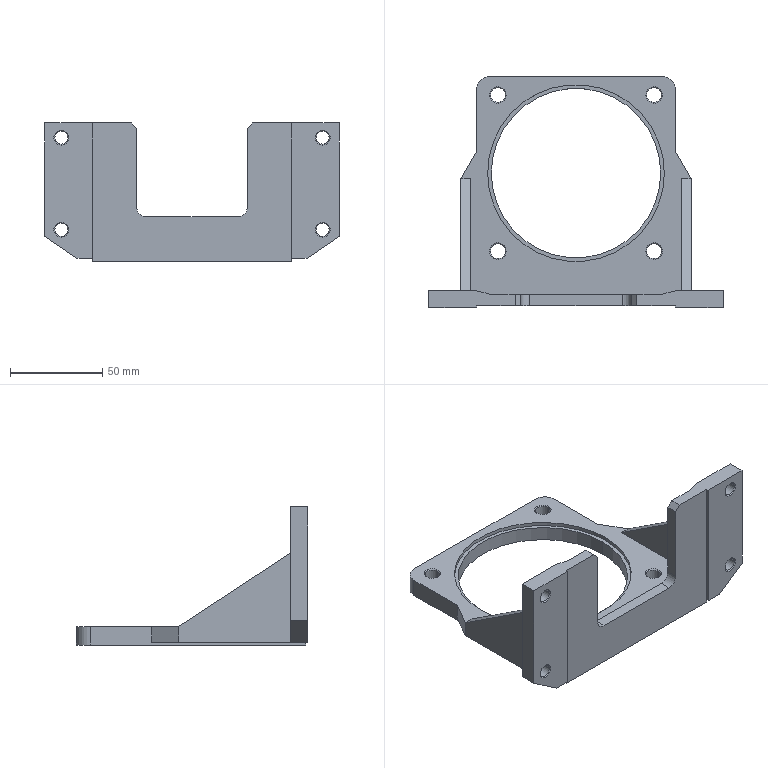Part | STEP file | DDK motor base (RAL100) | 1 solid | 93 faces | box 160 x 125.5 x 75 mm | volume 142443 mm3 | plane 37 | cone 32 | cylinder 24 | commonest cylinder face diameters 7 x8 8 x8 10 x2 15 x2 92 x2 96 x2